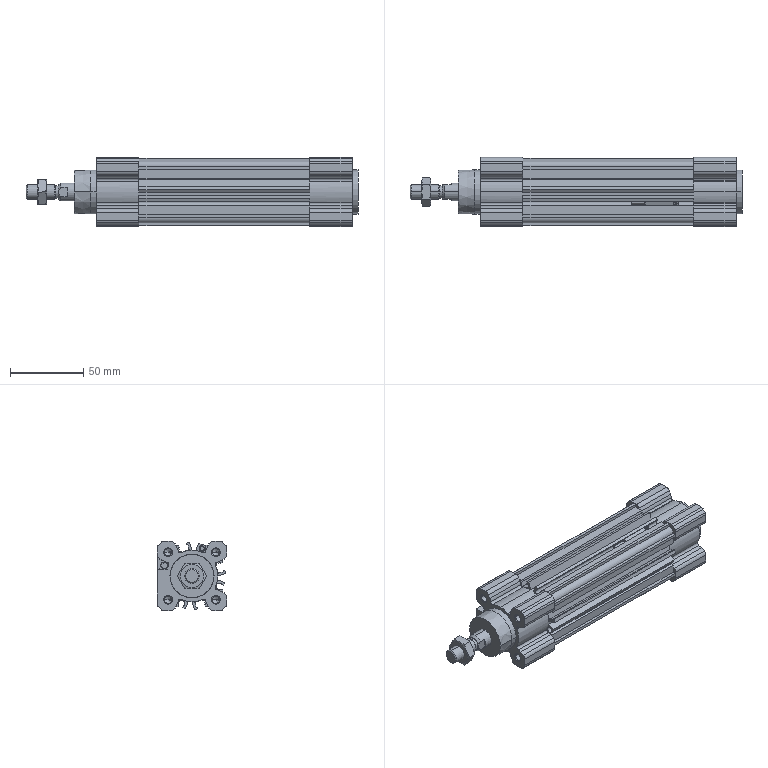Part | SolidWorks | 5 solids | 454 faces | box 226 x 47 x 47 mm | volume 241103 mm3 | plane 238 | cylinder 156 | cone 60 | commonest cylinder face diameters 6 x34 3 x18 4.917 x16 13.6 x14 4.25 x9 16.4 x8